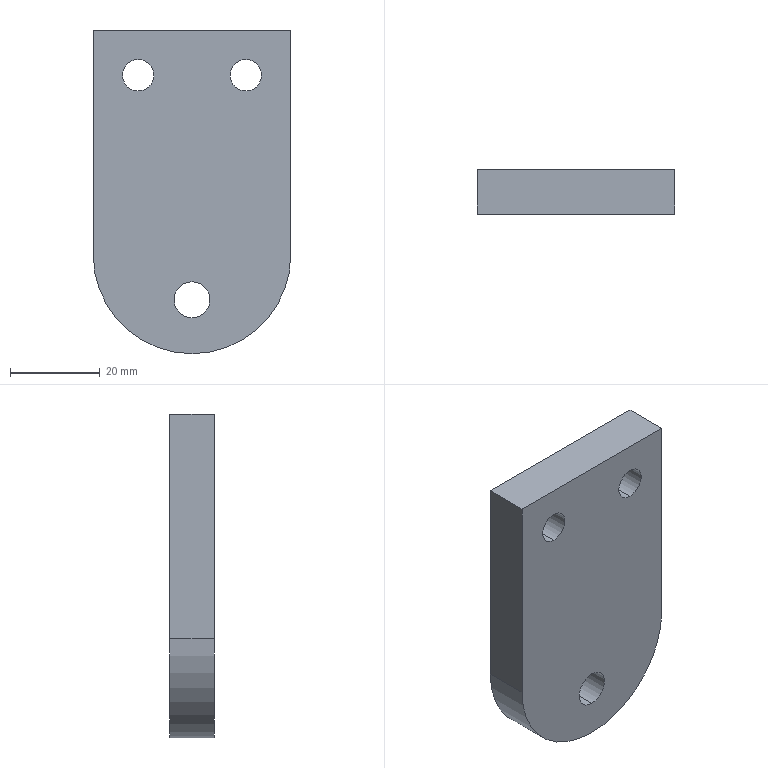Part | STEP file | OP10-146_seal side plate (1) | 1 solid | 13 faces | box 44 x 10 x 72 mm | volume 28330 mm3 | cylinder 8 | plane 5 | commonest cylinder face diameters 7 x4 8 x2 44 x2
STEP:
#1=CARTESIAN_POINT('',(0.,0.,0.));
#2=DIRECTION('',(0.,0.,1.));
#3=DIRECTION('',(1.,0.,0.));
#4=AXIS2_PLACEMENT_3D('',#1,#2,#3);
#5=CARTESIAN_POINT('',(12.,10.,-10.773));
#6=VERTEX_POINT('',#5);
#7=CARTESIAN_POINT('',(12.,0.,-10.773));
#8=VERTEX_POINT('',#7);
#9=CARTESIAN_POINT('',(12.,10.,-10.773));
#10=DIRECTION('',(0.,-1.,0.));
#11=VECTOR('',#10,1.);
#12=LINE('',#9,#11);
#13=CARTESIAN_POINT('',(12.,10.,-7.273));
#14=DIRECTION('',(0.,-1.,0.));
#15=DIRECTION('',(0.,0.,-1.));
#16=AXIS2_PLACEMENT_3D('',#13,#14,#15);
#17=CYLINDRICAL_SURFACE('',#16,3.5);
#18=CARTESIAN_POINT('',(6.283,0.));
#19=DIRECTION('',(0.,1.));
#20=VECTOR('',#19,1.);
#21=LINE('',#18,#20);
#22=(GEOMETRIC_REPRESENTATION_CONTEXT(2)PARAMETRIC_REPRESENTATION_CONTEXT()REPRESENTATION_CONTEXT('',''));
#23=DEFINITIONAL_REPRESENTATION('',(#21),#22);
#24=PCURVE('',#17,#23);
#25=CARTESIAN_POINT('',(12.,10.,-7.273));
#26=DIRECTION('',(0.,-1.,0.));
#27=DIRECTION('',(0.,0.,-1.));
#28=AXIS2_PLACEMENT_3D('',#25,#26,#27);
#29=CYLINDRICAL_SURFACE('',#28,3.5);
#30=CARTESIAN_POINT('',(0.,0.));
#31=DIRECTION('',(0.,1.));
#32=VECTOR('',#31,1.);
#33=LINE('',#30,#32);
#34=(GEOMETRIC_REPRESENTATION_CONTEXT(2)PARAMETRIC_REPRESENTATION_CONTEXT()REPRESENTATION_CONTEXT('',''));
#35=DEFINITIONAL_REPRESENTATION('',(#33),#34);
#36=PCURVE('',#29,#35);
#37=SURFACE_CURVE('',#12,(#24,#36),.PCURVE_S1.);
#38=EDGE_CURVE('',#6,#8,#37,.T.);
#39=ORIENTED_EDGE('',*,*,#38,.T.);
#40=CARTESIAN_POINT('',(12.,0.,-3.773));
#41=VERTEX_POINT('',#40);
#42=CARTESIAN_POINT('',(12.,0.,-7.273));
#43=DIRECTION('',(0.,1.,0.));
#44=DIRECTION('',(0.,0.,1.));
#45=AXIS2_PLACEMENT_3D('',#42,#43,#44);
#46=CIRCLE('',#45,3.5);
#47=CARTESIAN_POINT('',(9.425,10.));
#48=DIRECTION('',(-1.,0.));
#49=VECTOR('',#48,1.);
#50=LINE('',#47,#49);
#51=(GEOMETRIC_REPRESENTATION_CONTEXT(2)PARAMETRIC_REPRESENTATION_CONTEXT()REPRESENTATION_CONTEXT('',''));
#52=DEFINITIONAL_REPRESENTATION('',(#50),#51);
#53=PCURVE('',#17,#52);
#54=CARTESIAN_POINT('',(0.,0.,-47.273));
#55=DIRECTION('',(0.,1.,0.));
#56=DIRECTION('',(0.,0.,1.));
#57=AXIS2_PLACEMENT_3D('',#54,#55,#56);
#58=PLANE('',#57);
#59=CARTESIAN_POINT('',(40.,12.));
#60=DIRECTION('',(1.,0.));
#61=AXIS2_PLACEMENT_2D('',#59,#60);
#62=CIRCLE('',#61,3.5);
#63=(GEOMETRIC_REPRESENTATION_CONTEXT(2)PARAMETRIC_REPRESENTATION_CONTEXT()REPRESENTATION_CONTEXT('',''));
#64=DEFINITIONAL_REPRESENTATION('',(#62),#63);
#65=PCURVE('',#58,#64);
#66=SURFACE_CURVE('',#46,(#53,#65),.PCURVE_S1.);
#67=EDGE_CURVE('',#8,#41,#66,.T.);
#68=ORIENTED_EDGE('',*,*,#67,.T.);
#69=CARTESIAN_POINT('',(12.,10.,-3.773));
#70=VERTEX_POINT('',#69);
#71=CARTESIAN_POINT('',(12.,10.,-3.773));
#72=DIRECTION('',(0.,-1.,0.));
#73=VECTOR('',#72,1.);
#74=LINE('',#71,#73);
#75=CARTESIAN_POINT('',(3.142,0.));
#76=DIRECTION('',(0.,1.));
#77=VECTOR('',#76,1.);
#78=LINE('',#75,#77);
#79=(GEOMETRIC_REPRESENTATION_CONTEXT(2)PARAMETRIC_REPRESENTATION_CONTEXT()REPRESENTATION_CONTEXT('',''));
#80=DEFINITIONAL_REPRESENTATION('',(#78),#79);
#81=PCURVE('',#17,#80);
#82=CARTESIAN_POINT('',(3.142,0.));
#83=DIRECTION('',(0.,1.));
#84=VECTOR('',#83,1.);
#85=LINE('',#82,#84);
#86=(GEOMETRIC_REPRESENTATION_CONTEXT(2)PARAMETRIC_REPRESENTATION_CONTEXT()REPRESENTATION_CONTEXT('',''));
#87=DEFINITIONAL_REPRESENTATION('',(#85),#86);
#88=PCURVE('',#29,#87);
#89=SURFACE_CURVE('',#74,(#81,#88),.PCURVE_S1.);
#90=EDGE_CURVE('',#70,#41,#89,.T.);
#91=ORIENTED_EDGE('',*,*,#90,.F.);
#92=CARTESIAN_POINT('',(12.,10.,-7.273));
#93=DIRECTION('',(0.,1.,0.));
#94=DIRECTION('',(0.,0.,1.));
#95=AXIS2_PLACEMENT_3D('',#92,#93,#94);
#96=CIRCLE('',#95,3.5);
#97=CARTESIAN_POINT('',(9.425,0.));
#98=DIRECTION('',(-1.,0.));
#99=VECTOR('',#98,1.);
#100=LINE('',#97,#99);
#101=(GEOMETRIC_REPRESENTATION_CONTEXT(2)PARAMETRIC_REPRESENTATION_CONTEXT()REPRESENTATION_CONTEXT('',''));
#102=DEFINITIONAL_REPRESENTATION('',(#100),#101);
#103=PCURVE('',#17,#102);
#104=CARTESIAN_POINT('',(0.,10.,-47.273));
#105=DIRECTION('',(0.,1.,0.));
#106=DIRECTION('',(0.,0.,1.));
#107=AXIS2_PLACEMENT_3D('',#104,#105,#106);
#108=PLANE('',#107);
#109=CARTESIAN_POINT('',(40.,12.));
#110=DIRECTION('',(1.,0.));
#111=AXIS2_PLACEMENT_2D('',#109,#110);
#112=CIRCLE('',#111,3.5);
#113=(GEOMETRIC_REPRESENTATION_CONTEXT(2)PARAMETRIC_REPRESENTATION_CONTEXT()REPRESENTATION_CONTEXT('',''));
#114=DEFINITIONAL_REPRESENTATION('',(#112),#113);
#115=PCURVE('',#108,#114);
#116=SURFACE_CURVE('',#96,(#103,#115),.PCURVE_S1.);
#117=EDGE_CURVE('',#6,#70,#116,.T.);
#118=ORIENTED_EDGE('',*,*,#117,.F.);
#119=EDGE_LOOP('',(#39,#68,#91,#118));
#120=FACE_BOUND('',#119,.F.);
#121=ADVANCED_FACE('',(#120),#17,.F.);
#122=CARTESIAN_POINT('',(-12.,10.,-10.773));
#123=VERTEX_POINT('',#122);
#124=CARTESIAN_POINT('',(-12.,0.,-10.773));
#125=VERTEX_POINT('',#124);
#126=CARTESIAN_POINT('',(-12.,10.,-10.773));
#127=DIRECTION('',(0.,-1.,0.));
#128=VECTOR('',#127,1.);
#129=LINE('',#126,#128);
#130=CARTESIAN_POINT('',(-12.,10.,-7.273));
#131=DIRECTION('',(0.,-1.,0.));
#132=DIRECTION('',(0.,0.,-1.));
#133=AXIS2_PLACEMENT_3D('',#130,#131,#132);
#134=CYLINDRICAL_SURFACE('',#133,3.5);
#135=CARTESIAN_POINT('',(6.283,0.));
#136=DIRECTION('',(0.,1.));
#137=VECTOR('',#136,1.);
#138=LINE('',#135,#137);
#139=(GEOMETRIC_REPRESENTATION_CONTEXT(2)PARAMETRIC_REPRESENTATION_CONTEXT()REPRESENTATION_CONTEXT('',''));
#140=DEFINITIONAL_REPRESENTATION('',(#138),#139);
#141=PCURVE('',#134,#140);
#142=CARTESIAN_POINT('',(-12.,10.,-7.273));
#143=DIRECTION('',(0.,-1.,0.));
#144=DIRECTION('',(0.,0.,-1.));
#145=AXIS2_PLACEMENT_3D('',#142,#143,#144);
#146=CYLINDRICAL_SURFACE('',#145,3.5);
#147=CARTESIAN_POINT('',(0.,0.));
#148=DIRECTION('',(0.,1.));
#149=VECTOR('',#148,1.);
#150=LINE('',#147,#149);
#151=(GEOMETRIC_REPRESENTATION_CONTEXT(2)PARAMETRIC_REPRESENTATION_CONTEXT()REPRESENTATION_CONTEXT('',''));
#152=DEFINITIONAL_REPRESENTATION('',(#150),#151);
#153=PCURVE('',#146,#152);
#154=SURFACE_CURVE('',#129,(#141,#153),.PCURVE_S1.);
#155=EDGE_CURVE('',#123,#125,#154,.T.);
#156=ORIENTED_EDGE('',*,*,#155,.T.);
#157=CARTESIAN_POINT('',(-12.,0.,-3.773));
#158=VERTEX_POINT('',#157);
#159=CARTESIAN_POINT('',(-12.,0.,-7.273));
#160=DIRECTION('',(0.,1.,0.));
#161=DIRECTION('',(0.,0.,1.));
#162=AXIS2_PLACEMENT_3D('',#159,#160,#161);
#163=CIRCLE('',#162,3.5);
#164=CARTESIAN_POINT('',(9.425,10.));
#165=DIRECTION('',(-1.,0.));
#166=VECTOR('',#165,1.);
#167=LINE('',#164,#166);
#168=(GEOMETRIC_REPRESENTATION_CONTEXT(2)PARAMETRIC_REPRESENTATION_CONTEXT()REPRESENTATION_CONTEXT('',''));
#169=DEFINITIONAL_REPRESENTATION('',(#167),#168);
#170=PCURVE('',#134,#169);
#171=CARTESIAN_POINT('',(40.,-12.));
#172=DIRECTION('',(1.,0.));
#173=AXIS2_PLACEMENT_2D('',#171,#172);
#174=CIRCLE('',#173,3.5);
#175=(GEOMETRIC_REPRESENTATION_CONTEXT(2)PARAMETRIC_REPRESENTATION_CONTEXT()REPRESENTATION_CONTEXT('',''));
#176=DEFINITIONAL_REPRESENTATION('',(#174),#175);
#177=PCURVE('',#58,#176);
#178=SURFACE_CURVE('',#163,(#170,#177),.PCURVE_S1.);
#179=EDGE_CURVE('',#125,#158,#178,.T.);
#180=ORIENTED_EDGE('',*,*,#179,.T.);
#181=CARTESIAN_POINT('',(-12.,10.,-3.773));
#182=VERTEX_POINT('',#181);
#183=CARTESIAN_POINT('',(-12.,10.,-3.773));
#184=DIRECTION('',(0.,-1.,0.));
#185=VECTOR('',#184,1.);
#186=LINE('',#183,#185);
#187=CARTESIAN_POINT('',(3.142,0.));
#188=DIRECTION('',(0.,1.));
#189=VECTOR('',#188,1.);
#190=LINE('',#187,#189);
#191=(GEOMETRIC_REPRESENTATION_CONTEXT(2)PARAMETRIC_REPRESENTATION_CONTEXT()REPRESENTATION_CONTEXT('',''));
#192=DEFINITIONAL_REPRESENTATION('',(#190),#191);
#193=PCURVE('',#134,#192);
#194=CARTESIAN_POINT('',(3.142,0.));
#195=DIRECTION('',(0.,1.));
#196=VECTOR('',#195,1.);
#197=LINE('',#194,#196);
#198=(GEOMETRIC_REPRESENTATION_CONTEXT(2)PARAMETRIC_REPRESENTATION_CONTEXT()REPRESENTATION_CONTEXT('',''));
#199=DEFINITIONAL_REPRESENTATION('',(#197),#198);
#200=PCURVE('',#146,#199);
#201=SURFACE_CURVE('',#186,(#193,#200),.PCURVE_S1.);
#202=EDGE_CURVE('',#182,#158,#201,.T.);
#203=ORIENTED_EDGE('',*,*,#202,.F.);
#204=CARTESIAN_POINT('',(-12.,10.,-7.273));
#205=DIRECTION('',(0.,1.,0.));
#206=DIRECTION('',(0.,0.,1.));
#207=AXIS2_PLACEMENT_3D('',#204,#205,#206);
#208=CIRCLE('',#207,3.5);
#209=CARTESIAN_POINT('',(9.425,0.));
#210=DIRECTION('',(-1.,0.));
#211=VECTOR('',#210,1.);
#212=LINE('',#209,#211);
#213=(GEOMETRIC_REPRESENTATION_CONTEXT(2)PARAMETRIC_REPRESENTATION_CONTEXT()REPRESENTATION_CONTEXT('',''));
#214=DEFINITIONAL_REPRESENTATION('',(#212),#213);
#215=PCURVE('',#134,#214);
#216=CARTESIAN_POINT('',(40.,-12.));
#217=DIRECTION('',(1.,0.));
#218=AXIS2_PLACEMENT_2D('',#216,#217);
#219=CIRCLE('',#218,3.5);
#220=(GEOMETRIC_REPRESENTATION_CONTEXT(2)PARAMETRIC_REPRESENTATION_CONTEXT()REPRESENTATION_CONTEXT('',''));
#221=DEFINITIONAL_REPRESENTATION('',(#219),#220);
#222=PCURVE('',#108,#221);
#223=SURFACE_CURVE('',#208,(#215,#222),.PCURVE_S1.);
#224=EDGE_CURVE('',#123,#182,#223,.T.);
#225=ORIENTED_EDGE('',*,*,#224,.F.);
#226=EDGE_LOOP('',(#156,#180,#203,#225));
#227=FACE_BOUND('',#226,.F.);
#228=ADVANCED_FACE('',(#227),#134,.F.);
#229=CARTESIAN_POINT('',(0.,10.,-61.273));
#230=VERTEX_POINT('',#229);
#231=CARTESIAN_POINT('',(0.,0.,-61.273));
#232=VERTEX_POINT('',#231);
#233=CARTESIAN_POINT('',(0.,10.,-61.273));
#234=DIRECTION('',(0.,-1.,0.));
#235=VECTOR('',#234,1.);
#236=LINE('',#233,#235);
#237=CARTESIAN_POINT('',(0.,10.,-57.273));
#238=DIRECTION('',(0.,-1.,0.));
#239=DIRECTION('',(0.,0.,-1.));
#240=AXIS2_PLACEMENT_3D('',#237,#238,#239);
#241=CYLINDRICAL_SURFACE('',#240,4.);
#242=CARTESIAN_POINT('',(6.283,0.));
#243=DIRECTION('',(0.,1.));
#244=VECTOR('',#243,1.);
#245=LINE('',#242,#244);
#246=(GEOMETRIC_REPRESENTATION_CONTEXT(2)PARAMETRIC_REPRESENTATION_CONTEXT()REPRESENTATION_CONTEXT('',''));
#247=DEFINITIONAL_REPRESENTATION('',(#245),#246);
#248=PCURVE('',#241,#247);
#249=CARTESIAN_POINT('',(0.,10.,-57.273));
#250=DIRECTION('',(0.,-1.,0.));
#251=DIRECTION('',(0.,0.,-1.));
#252=AXIS2_PLACEMENT_3D('',#249,#250,#251);
#253=CYLINDRICAL_SURFACE('',#252,4.);
#254=CARTESIAN_POINT('',(0.,0.));
#255=DIRECTION('',(0.,1.));
#256=VECTOR('',#255,1.);
#257=LINE('',#254,#256);
#258=(GEOMETRIC_REPRESENTATION_CONTEXT(2)PARAMETRIC_REPRESENTATION_CONTEXT()REPRESENTATION_CONTEXT('',''));
#259=DEFINITIONAL_REPRESENTATION('',(#257),#258);
#260=PCURVE('',#253,#259);
#261=SURFACE_CURVE('',#236,(#248,#260),.PCURVE_S1.);
#262=EDGE_CURVE('',#230,#232,#261,.T.);
#263=ORIENTED_EDGE('',*,*,#262,.T.);
#264=CARTESIAN_POINT('',(0.,0.,-53.273));
#265=VERTEX_POINT('',#264);
#266=CARTESIAN_POINT('',(0.,0.,-57.273));
#267=DIRECTION('',(0.,1.,0.));
#268=DIRECTION('',(0.,0.,1.));
#269=AXIS2_PLACEMENT_3D('',#266,#267,#268);
#270=CIRCLE('',#269,4.);
#271=CARTESIAN_POINT('',(9.425,10.));
#272=DIRECTION('',(-1.,0.));
#273=VECTOR('',#272,1.);
#274=LINE('',#271,#273);
#275=(GEOMETRIC_REPRESENTATION_CONTEXT(2)PARAMETRIC_REPRESENTATION_CONTEXT()REPRESENTATION_CONTEXT('',''));
#276=DEFINITIONAL_REPRESENTATION('',(#274),#275);
#277=PCURVE('',#241,#276);
#278=CARTESIAN_POINT('',(-10.,0.));
#279=DIRECTION('',(1.,0.));
#280=AXIS2_PLACEMENT_2D('',#278,#279);
#281=CIRCLE('',#280,4.);
#282=(GEOMETRIC_REPRESENTATION_CONTEXT(2)PARAMETRIC_REPRESENTATION_CONTEXT()REPRESENTATION_CONTEXT('',''));
#283=DEFINITIONAL_REPRESENTATION('',(#281),#282);
#284=PCURVE('',#58,#283);
#285=SURFACE_CURVE('',#270,(#277,#284),.PCURVE_S1.);
#286=EDGE_CURVE('',#232,#265,#285,.T.);
#287=ORIENTED_EDGE('',*,*,#286,.T.);
#288=CARTESIAN_POINT('',(0.,10.,-53.273));
#289=VERTEX_POINT('',#288);
#290=CARTESIAN_POINT('',(0.,10.,-53.273));
#291=DIRECTION('',(0.,-1.,0.));
#292=VECTOR('',#291,1.);
#293=LINE('',#290,#292);
#294=CARTESIAN_POINT('',(3.142,0.));
#295=DIRECTION('',(0.,1.));
#296=VECTOR('',#295,1.);
#297=LINE('',#294,#296);
#298=(GEOMETRIC_REPRESENTATION_CONTEXT(2)PARAMETRIC_REPRESENTATION_CONTEXT()REPRESENTATION_CONTEXT('',''));
#299=DEFINITIONAL_REPRESENTATION('',(#297),#298);
#300=PCURVE('',#241,#299);
#301=CARTESIAN_POINT('',(3.142,0.));
#302=DIRECTION('',(0.,1.));
#303=VECTOR('',#302,1.);
#304=LINE('',#301,#303);
#305=(GEOMETRIC_REPRESENTATION_CONTEXT(2)PARAMETRIC_REPRESENTATION_CONTEXT()REPRESENTATION_CONTEXT('',''));
#306=DEFINITIONAL_REPRESENTATION('',(#304),#305);
#307=PCURVE('',#253,#306);
#308=SURFACE_CURVE('',#293,(#300,#307),.PCURVE_S1.);
#309=EDGE_CURVE('',#289,#265,#308,.T.);
#310=ORIENTED_EDGE('',*,*,#309,.F.);
#311=CARTESIAN_POINT('',(0.,10.,-57.273));
#312=DIRECTION('',(0.,1.,0.));
#313=DIRECTION('',(0.,0.,1.));
#314=AXIS2_PLACEMENT_3D('',#311,#312,#313);
#315=CIRCLE('',#314,4.);
#316=CARTESIAN_POINT('',(9.425,0.));
#317=DIRECTION('',(-1.,0.));
#318=VECTOR('',#317,1.);
#319=LINE('',#316,#318);
#320=(GEOMETRIC_REPRESENTATION_CONTEXT(2)PARAMETRIC_REPRESENTATION_CONTEXT()REPRESENTATION_CONTEXT('',''));
#321=DEFINITIONAL_REPRESENTATION('',(#319),#320);
#322=PCURVE('',#241,#321);
#323=CARTESIAN_POINT('',(-10.,0.));
#324=DIRECTION('',(1.,0.));
#325=AXIS2_PLACEMENT_2D('',#323,#324);
#326=CIRCLE('',#325,4.);
#327=(GEOMETRIC_REPRESENTATION_CONTEXT(2)PARAMETRIC_REPRESENTATION_CONTEXT()REPRESENTATION_CONTEXT('',''));
#328=DEFINITIONAL_REPRESENTATION('',(#326),#327);
#329=PCURVE('',#108,#328);
#330=SURFACE_CURVE('',#315,(#322,#329),.PCURVE_S1.);
#331=EDGE_CURVE('',#230,#289,#330,.T.);
#332=ORIENTED_EDGE('',*,*,#331,.F.);
#333=EDGE_LOOP('',(#263,#287,#310,#332));
#334=FACE_BOUND('',#333,.F.);
#335=ADVANCED_FACE('',(#334),#241,.F.);
#336=CARTESIAN_POINT('',(0.,10.,-69.273));
#337=VERTEX_POINT('',#336);
#338=CARTESIAN_POINT('',(-22.,10.,-47.273));
#339=VERTEX_POINT('',#338);
#340=CARTESIAN_POINT('',(0.,10.,-47.273));
#341=DIRECTION('',(0.,1.,0.));
#342=DIRECTION('',(0.,0.,1.));
#343=AXIS2_PLACEMENT_3D('',#340,#341,#342);
#344=CIRCLE('',#343,22.);
#345=CARTESIAN_POINT('',(0.,10.,-47.273));
#346=DIRECTION('',(0.,-1.,0.));
#347=DIRECTION('',(0.,0.,-1.));
#348=AXIS2_PLACEMENT_3D('',#345,#346,#347);
#349=CYLINDRICAL_SURFACE('',#348,22.);
#350=CARTESIAN_POINT('',(9.425,0.));
#351=DIRECTION('',(-1.,0.));
#352=VECTOR('',#351,1.);
#353=LINE('',#350,#352);
#354=(GEOMETRIC_REPRESENTATION_CONTEXT(2)PARAMETRIC_REPRESENTATION_CONTEXT()REPRESENTATION_CONTEXT('',''));
#355=DEFINITIONAL_REPRESENTATION('',(#353),#354);
#356=PCURVE('',#349,#355);
#357=CARTESIAN_POINT('',(0.,0.));
#358=DIRECTION('',(1.,0.));
#359=AXIS2_PLACEMENT_2D('',#357,#358);
#360=CIRCLE('',#359,22.);
#361=(GEOMETRIC_REPRESENTATION_CONTEXT(2)PARAMETRIC_REPRESENTATION_CONTEXT()REPRESENTATION_CONTEXT('',''));
#362=DEFINITIONAL_REPRESENTATION('',(#360),#361);
#363=PCURVE('',#108,#362);
#364=SURFACE_CURVE('',#344,(#356,#363),.PCURVE_S1.);
#365=EDGE_CURVE('',#337,#339,#364,.T.);
#366=ORIENTED_EDGE('',*,*,#365,.F.);
#367=CARTESIAN_POINT('',(0.,0.,-69.273));
#368=VERTEX_POINT('',#367);
#369=CARTESIAN_POINT('',(0.,10.,-69.273));
#370=DIRECTION('',(0.,-1.,0.));
#371=VECTOR('',#370,1.);
#372=LINE('',#369,#371);
#373=CARTESIAN_POINT('',(6.283,0.));
#374=DIRECTION('',(0.,1.));
#375=VECTOR('',#374,1.);
#376=LINE('',#373,#375);
#377=(GEOMETRIC_REPRESENTATION_CONTEXT(2)PARAMETRIC_REPRESENTATION_CONTEXT()REPRESENTATION_CONTEXT('',''));
#378=DEFINITIONAL_REPRESENTATION('',(#376),#377);
#379=PCURVE('',#349,#378);
#380=CARTESIAN_POINT('',(0.,10.,-47.273));
#381=DIRECTION('',(0.,-1.,0.));
#382=DIRECTION('',(0.,0.,-1.));
#383=AXIS2_PLACEMENT_3D('',#380,#381,#382);
#384=CYLINDRICAL_SURFACE('',#383,22.);
#385=CARTESIAN_POINT('',(0.,0.));
#386=DIRECTION('',(0.,1.));
#387=VECTOR('',#386,1.);
#388=LINE('',#385,#387);
#389=(GEOMETRIC_REPRESENTATION_CONTEXT(2)PARAMETRIC_REPRESENTATION_CONTEXT()REPRESENTATION_CONTEXT('',''));
#390=DEFINITIONAL_REPRESENTATION('',(#388),#389);
#391=PCURVE('',#384,#390);
#392=SURFACE_CURVE('',#372,(#379,#391),.PCURVE_S1.);
#393=EDGE_CURVE('',#337,#368,#392,.T.);
#394=ORIENTED_EDGE('',*,*,#393,.T.);
#395=CARTESIAN_POINT('',(-22.,0.,-47.273));
#396=VERTEX_POINT('',#395);
#397=CARTESIAN_POINT('',(0.,0.,-47.273));
#398=DIRECTION('',(0.,1.,0.));
#399=DIRECTION('',(0.,0.,1.));
#400=AXIS2_PLACEMENT_3D('',#397,#398,#399);
#401=CIRCLE('',#400,22.);
#402=CARTESIAN_POINT('',(9.425,10.));
#403=DIRECTION('',(-1.,0.));
#404=VECTOR('',#403,1.);
#405=LINE('',#402,#404);
#406=(GEOMETRIC_REPRESENTATION_CONTEXT(2)PARAMETRIC_REPRESENTATION_CONTEXT()REPRESENTATION_CONTEXT('',''));
#407=DEFINITIONAL_REPRESENTATION('',(#405),#406);
#408=PCURVE('',#349,#407);
#409=CARTESIAN_POINT('',(0.,0.));
#410=DIRECTION('',(1.,0.));
#411=AXIS2_PLACEMENT_2D('',#409,#410);
#412=CIRCLE('',#411,22.);
#413=(GEOMETRIC_REPRESENTATION_CONTEXT(2)PARAMETRIC_REPRESENTATION_CONTEXT()REPRESENTATION_CONTEXT('',''));
#414=DEFINITIONAL_REPRESENTATION('',(#412),#413);
#415=PCURVE('',#58,#414);
#416=SURFACE_CURVE('',#401,(#408,#415),.PCURVE_S1.);
#417=EDGE_CURVE('',#368,#396,#416,.T.);
#418=ORIENTED_EDGE('',*,*,#417,.T.);
#419=CARTESIAN_POINT('',(-22.,10.,-47.273));
#420=DIRECTION('',(0.,-1.,0.));
#421=VECTOR('',#420,1.);
#422=LINE('',#419,#421);
#423=CARTESIAN_POINT('',(4.712,0.));
#424=DIRECTION('',(0.,1.));
#425=VECTOR('',#424,1.);
#426=LINE('',#423,#425);
#427=(GEOMETRIC_REPRESENTATION_CONTEXT(2)PARAMETRIC_REPRESENTATION_CONTEXT()REPRESENTATION_CONTEXT('',''));
#428=DEFINITIONAL_REPRESENTATION('',(#426),#427);
#429=PCURVE('',#349,#428);
#430=CARTESIAN_POINT('',(-22.,10.,2.727));
#431=DIRECTION('',(1.,0.,0.));
#432=DIRECTION('',(0.,0.,-1.));
#433=AXIS2_PLACEMENT_3D('',#430,#431,#432);
#434=PLANE('',#433);
#435=CARTESIAN_POINT('',(50.,0.));
#436=DIRECTION('',(0.,-1.));
#437=VECTOR('',#436,1.);
#438=LINE('',#435,#437);
#439=(GEOMETRIC_REPRESENTATION_CONTEXT(2)PARAMETRIC_REPRESENTATION_CONTEXT()REPRESENTATION_CONTEXT('',''));
#440=DEFINITIONAL_REPRESENTATION('',(#438),#439);
#441=PCURVE('',#434,#440);
#442=SURFACE_CURVE('',#422,(#429,#441),.PCURVE_S1.);
#443=EDGE_CURVE('',#339,#396,#442,.T.);
#444=ORIENTED_EDGE('',*,*,#443,.F.);
#445=EDGE_LOOP('',(#366,#394,#418,#444));
#446=FACE_BOUND('',#445,.T.);
#447=ADVANCED_FACE('',(#446),#349,.T.);
#448=ORIENTED_EDGE('',*,*,#224,.F.);
#449=CARTESIAN_POINT('',(-12.,10.,-7.273));
#450=DIRECTION('',(0.,1.,0.));
#451=DIRECTION('',(0.,0.,1.));
#452=AXIS2_PLACEMENT_3D('',#449,#450,#451);
#453=CIRCLE('',#452,3.5);
#454=CARTESIAN_POINT('',(40.,-12.));
#455=DIRECTION('',(1.,0.));
#456=AXIS2_PLACEMENT_2D('',#454,#455);
#457=CIRCLE('',#456,3.5);
#458=(GEOMETRIC_REPRESENTATION_CONTEXT(2)PARAMETRIC_REPRESENTATION_CONTEXT()REPRESENTATION_CONTEXT('',''));
#459=DEFINITIONAL_REPRESENTATION('',(#457),#458);
#460=PCURVE('',#108,#459);
#461=CARTESIAN_POINT('',(3.142,0.));
#462=DIRECTION('',(-1.,0.));
#463=VECTOR('',#462,1.);
#464=LINE('',#461,#463);
#465=(GEOMETRIC_REPRESENTATION_CONTEXT(2)PARAMETRIC_REPRESENTATION_CONTEXT()REPRESENTATION_CONTEXT('',''));
#466=DEFINITIONAL_REPRESENTATION('',(#464),#465);
#467=PCURVE('',#146,#466);
#468=SURFACE_CURVE('',#453,(#460,#467),.PCURVE_S1.);
#469=EDGE_CURVE('',#182,#123,#468,.T.);
#470=ORIENTED_EDGE('',*,*,#469,.F.);
#471=EDGE_LOOP('',(#448,#470));
#472=FACE_BOUND('',#471,.T.);
#473=CARTESIAN_POINT('',(22.,10.,-47.273));
#474=VERTEX_POINT('',#473);
#475=CARTESIAN_POINT('',(0.,10.,-47.273));
#476=DIRECTION('',(0.,1.,0.));
#477=DIRECTION('',(0.,0.,1.));
#478=AXIS2_PLACEMENT_3D('',#475,#476,#477);
#479=CIRCLE('',#478,22.);
#480=CARTESIAN_POINT('',(0.,0.));
#481=DIRECTION('',(1.,0.));
#482=AXIS2_PLACEMENT_2D('',#480,#481);
#483=CIRCLE('',#482,22.);
#484=(GEOMETRIC_REPRESENTATION_CONTEXT(2)PARAMETRIC_REPRESENTATION_CONTEXT()REPRESENTATION_CONTEXT('',''));
#485=DEFINITIONAL_REPRESENTATION('',(#483),#484);
#486=PCURVE('',#108,#485);
#487=CARTESIAN_POINT('',(3.142,0.));
#488=DIRECTION('',(-1.,0.));
#489=VECTOR('',#488,1.);
#490=LINE('',#487,#489);
#491=(GEOMETRIC_REPRESENTATION_CONTEXT(2)PARAMETRIC_REPRESENTATION_CONTEXT()REPRESENTATION_CONTEXT('',''));
#492=DEFINITIONAL_REPRESENTATION('',(#490),#491);
#493=PCURVE('',#384,#492);
#494=SURFACE_CURVE('',#479,(#486,#493),.PCURVE_S1.);
#495=EDGE_CURVE('',#474,#337,#494,.T.);
#496=ORIENTED_EDGE('',*,*,#495,.T.);
#497=ORIENTED_EDGE('',*,*,#365,.T.);
#498=CARTESIAN_POINT('',(-22.,10.,2.727));
#499=VERTEX_POINT('',#498);
#500=CARTESIAN_POINT('',(-22.,10.,2.727));
#501=DIRECTION('',(0.,0.,1.));
#502=VECTOR('',#501,1.);
#503=LINE('',#500,#502);
#504=CARTESIAN_POINT('',(50.,-22.));
#505=DIRECTION('',(1.,0.));
#506=VECTOR('',#505,1.);
#507=LINE('',#504,#506);
#508=(GEOMETRIC_REPRESENTATION_CONTEXT(2)PARAMETRIC_REPRESENTATION_CONTEXT()REPRESENTATION_CONTEXT('',''));
#509=DEFINITIONAL_REPRESENTATION('',(#507),#508);
#510=PCURVE('',#108,#509);
#511=CARTESIAN_POINT('',(0.,0.));
#512=DIRECTION('',(-1.,0.));
#513=VECTOR('',#512,1.);
#514=LINE('',#511,#513);
#515=(GEOMETRIC_REPRESENTATION_CONTEXT(2)PARAMETRIC_REPRESENTATION_CONTEXT()REPRESENTATION_CONTEXT('',''));
#516=DEFINITIONAL_REPRESENTATION('',(#514),#515);
#517=PCURVE('',#434,#516);
#518=SURFACE_CURVE('',#503,(#510,#517),.PCURVE_S1.);
#519=EDGE_CURVE('',#339,#499,#518,.T.);
#520=ORIENTED_EDGE('',*,*,#519,.T.);
#521=CARTESIAN_POINT('',(22.,10.,2.727));
#522=VERTEX_POINT('',#521);
#523=CARTESIAN_POINT('',(-22.,10.,2.727));
#524=DIRECTION('',(1.,0.,0.));
#525=VECTOR('',#524,1.);
#526=LINE('',#523,#525);
#527=CARTESIAN_POINT('',(50.,-22.));
#528=DIRECTION('',(0.,1.));
#529=VECTOR('',#528,1.);
#530=LINE('',#527,#529);
#531=(GEOMETRIC_REPRESENTATION_CONTEXT(2)PARAMETRIC_REPRESENTATION_CONTEXT()REPRESENTATION_CONTEXT('',''));
#532=DEFINITIONAL_REPRESENTATION('',(#530),#531);
#533=PCURVE('',#108,#532);
#534=CARTESIAN_POINT('',(-22.,10.,2.727));
#535=DIRECTION('',(0.,0.,-1.));
#536=DIRECTION('',(-1.,0.,0.));
#537=AXIS2_PLACEMENT_3D('',#534,#535,#536);
#538=PLANE('',#537);
#539=CARTESIAN_POINT('',(0.,0.));
#540=DIRECTION('',(-1.,0.));
#541=VECTOR('',#540,1.);
#542=LINE('',#539,#541);
#543=(GEOMETRIC_REPRESENTATION_CONTEXT(2)PARAMETRIC_REPRESENTATION_CONTEXT()REPRESENTATION_CONTEXT('',''));
#544=DEFINITIONAL_REPRESENTATION('',(#542),#543);
#545=PCURVE('',#538,#544);
#546=SURFACE_CURVE('',#526,(#533,#545),.PCURVE_S1.);
#547=EDGE_CURVE('',#499,#522,#546,.T.);
#548=ORIENTED_EDGE('',*,*,#547,.T.);
#549=CARTESIAN_POINT('',(22.,10.,2.727));
#550=DIRECTION('',(0.,0.,-1.));
#551=VECTOR('',#550,1.);
#552=LINE('',#549,#551);
#553=CARTESIAN_POINT('',(50.,22.));
#554=DIRECTION('',(-1.,0.));
#555=VECTOR('',#554,1.);
#556=LINE('',#553,#555);
#557=(GEOMETRIC_REPRESENTATION_CONTEXT(2)PARAMETRIC_REPRESENTATION_CONTEXT()REPRESENTATION_CONTEXT('',''));
#558=DEFINITIONAL_REPRESENTATION('',(#556),#557);
#559=PCURVE('',#108,#558);
#560=CARTESIAN_POINT('',(22.,10.,2.727));
#561=DIRECTION('',(-1.,0.,0.));
#562=DIRECTION('',(0.,0.,1.));
#563=AXIS2_PLACEMENT_3D('',#560,#561,#562);
#564=PLANE('',#563);
#565=CARTESIAN_POINT('',(0.,0.));
#566=DIRECTION('',(-1.,0.));
#567=VECTOR('',#566,1.);
#568=LINE('',#565,#567);
#569=(GEOMETRIC_REPRESENTATION_CONTEXT(2)PARAMETRIC_REPRESENTATION_CONTEXT()REPRESENTATION_CONTEXT('',''));
#570=DEFINITIONAL_REPRESENTATION('',(#568),#569);
#571=PCURVE('',#564,#570);
#572=SURFACE_CURVE('',#552,(#559,#571),.PCURVE_S1.);
#573=EDGE_CURVE('',#522,#474,#572,.T.);
#574=ORIENTED_EDGE('',*,*,#573,.T.);
#575=EDGE_LOOP('',(#496,#497,#520,#548,#574));
#576=FACE_BOUND('',#575,.T.);
#577=ORIENTED_EDGE('',*,*,#331,.F.);
#578=CARTESIAN_POINT('',(0.,10.,-57.273));
#579=DIRECTION('',(0.,1.,0.));
#580=DIRECTION('',(0.,0.,1.));
#581=AXIS2_PLACEMENT_3D('',#578,#579,#580);
#582=CIRCLE('',#581,4.);
#583=CARTESIAN_POINT('',(-10.,0.));
#584=DIRECTION('',(1.,0.));
#585=AXIS2_PLACEMENT_2D('',#583,#584);
#586=CIRCLE('',#585,4.);
#587=(GEOMETRIC_REPRESENTATION_CONTEXT(2)PARAMETRIC_REPRESENTATION_CONTEXT()REPRESENTATION_CONTEXT('',''));
#588=DEFINITIONAL_REPRESENTATION('',(#586),#587);
#589=PCURVE('',#108,#588);
#590=CARTESIAN_POINT('',(3.142,0.));
#591=DIRECTION('',(-1.,0.));
#592=VECTOR('',#591,1.);
#593=LINE('',#590,#592);
#594=(GEOMETRIC_REPRESENTATION_CONTEXT(2)PARAMETRIC_REPRESENTATION_CONTEXT()REPRESENTATION_CONTEXT('',''));
#595=DEFINITIONAL_REPRESENTATION('',(#593),#594);
#596=PCURVE('',#253,#595);
#597=SURFACE_CURVE('',#582,(#589,#596),.PCURVE_S1.);
#598=EDGE_CURVE('',#289,#230,#597,.T.);
#599=ORIENTED_EDGE('',*,*,#598,.F.);
#600=EDGE_LOOP('',(#577,#599));
#601=FACE_BOUND('',#600,.T.);
#602=ORIENTED_EDGE('',*,*,#117,.F.);
#603=CARTESIAN_POINT('',(12.,10.,-7.273));
#604=DIRECTION('',(0.,1.,0.));
#605=DIRECTION('',(0.,0.,1.));
#606=AXIS2_PLACEMENT_3D('',#603,#604,#605);
#607=CIRCLE('',#606,3.5);
#608=CARTESIAN_POINT('',(40.,12.));
#609=DIRECTION('',(1.,0.));
#610=AXIS2_PLACEMENT_2D('',#608,#609);
#611=CIRCLE('',#610,3.5);
#612=(GEOMETRIC_REPRESENTATION_CONTEXT(2)PARAMETRIC_REPRESENTATION_CONTEXT()REPRESENTATION_CONTEXT('',''));
#613=DEFINITIONAL_REPRESENTATION('',(#611),#612);
#614=PCURVE('',#108,#613);
#615=CARTESIAN_POINT('',(3.142,0.));
#616=DIRECTION('',(-1.,0.));
#617=VECTOR('',#616,1.);
#618=LINE('',#615,#617);
#619=(GEOMETRIC_REPRESENTATION_CONTEXT(2)PARAMETRIC_REPRESENTATION_CONTEXT()REPRESENTATION_CONTEXT('',''));
#620=DEFINITIONAL_REPRESENTATION('',(#618),#619);
#621=PCURVE('',#29,#620);
#622=SURFACE_CURVE('',#607,(#614,#621),.PCURVE_S1.);
#623=EDGE_CURVE('',#70,#6,#622,.T.);
#624=ORIENTED_EDGE('',*,*,#623,.F.);
#625=EDGE_LOOP('',(#602,#624));
#626=FACE_BOUND('',#625,.T.);
#627=ADVANCED_FACE('',(#472,#576,#601,#626),#108,.T.);
#628=ORIENTED_EDGE('',*,*,#179,.T.);
#629=CARTESIAN_POINT('',(-12.,0.,-7.273));
#630=DIRECTION('',(0.,1.,0.));
#631=DIRECTION('',(0.,0.,1.));
#632=AXIS2_PLACEMENT_3D('',#629,#630,#631);
#633=CIRCLE('',#632,3.5);
#634=CARTESIAN_POINT('',(40.,-12.));
#635=DIRECTION('',(1.,0.));
#636=AXIS2_PLACEMENT_2D('',#634,#635);
#637=CIRCLE('',#636,3.5);
#638=(GEOMETRIC_REPRESENTATION_CONTEXT(2)PARAMETRIC_REPRESENTATION_CONTEXT()REPRESENTATION_CONTEXT('',''));
#639=DEFINITIONAL_REPRESENTATION('',(#637),#638);
#640=PCURVE('',#58,#639);
#641=CARTESIAN_POINT('',(3.142,10.));
#642=DIRECTION('',(-1.,0.));
#643=VECTOR('',#642,1.);
#644=LINE('',#641,#643);
#645=(GEOMETRIC_REPRESENTATION_CONTEXT(2)PARAMETRIC_REPRESENTATION_CONTEXT()REPRESENTATION_CONTEXT('',''));
#646=DEFINITIONAL_REPRESENTATION('',(#644),#645);
#647=PCURVE('',#146,#646);
#648=SURFACE_CURVE('',#633,(#640,#647),.PCURVE_S1.);
#649=EDGE_CURVE('',#158,#125,#648,.T.);
#650=ORIENTED_EDGE('',*,*,#649,.T.);
#651=EDGE_LOOP('',(#628,#650));
#652=FACE_BOUND('',#651,.T.);
#653=CARTESIAN_POINT('',(22.,0.,-47.273));
#654=VERTEX_POINT('',#653);
#655=CARTESIAN_POINT('',(0.,0.,-47.273));
#656=DIRECTION('',(0.,1.,0.));
#657=DIRECTION('',(0.,0.,1.));
#658=AXIS2_PLACEMENT_3D('',#655,#656,#657);
#659=CIRCLE('',#658,22.);
#660=CARTESIAN_POINT('',(0.,0.));
#661=DIRECTION('',(1.,0.));
#662=AXIS2_PLACEMENT_2D('',#660,#661);
#663=CIRCLE('',#662,22.);
#664=(GEOMETRIC_REPRESENTATION_CONTEXT(2)PARAMETRIC_REPRESENTATION_CONTEXT()REPRESENTATION_CONTEXT('',''));
#665=DEFINITIONAL_REPRESENTATION('',(#663),#664);
#666=PCURVE('',#58,#665);
#667=CARTESIAN_POINT('',(3.142,10.));
#668=DIRECTION('',(-1.,0.));
#669=VECTOR('',#668,1.);
#670=LINE('',#667,#669);
#671=(GEOMETRIC_REPRESENTATION_CONTEXT(2)PARAMETRIC_REPRESENTATION_CONTEXT()REPRESENTATION_CONTEXT('',''));
#672=DEFINITIONAL_REPRESENTATION('',(#670),#671);
#673=PCURVE('',#384,#672);
#674=SURFACE_CURVE('',#659,(#666,#673),.PCURVE_S1.);
#675=EDGE_CURVE('',#654,#368,#674,.T.);
#676=ORIENTED_EDGE('',*,*,#675,.F.);
#677=CARTESIAN_POINT('',(22.,0.,2.727));
#678=VERTEX_POINT('',#677);
#679=CARTESIAN_POINT('',(22.,0.,2.727));
#680=DIRECTION('',(0.,0.,-1.));
#681=VECTOR('',#680,1.);
#682=LINE('',#679,#681);
#683=CARTESIAN_POINT('',(50.,22.));
#684=DIRECTION('',(-1.,0.));
#685=VECTOR('',#684,1.);
#686=LINE('',#683,#685);
#687=(GEOMETRIC_REPRESENTATION_CONTEXT(2)PARAMETRIC_REPRESENTATION_CONTEXT()REPRESENTATION_CONTEXT('',''));
#688=DEFINITIONAL_REPRESENTATION('',(#686),#687);
#689=PCURVE('',#58,#688);
#690=CARTESIAN_POINT('',(0.,-10.));
#691=DIRECTION('',(-1.,0.));
#692=VECTOR('',#691,1.);
#693=LINE('',#690,#692);
#694=(GEOMETRIC_REPRESENTATION_CONTEXT(2)PARAMETRIC_REPRESENTATION_CONTEXT()REPRESENTATION_CONTEXT('',''));
#695=DEFINITIONAL_REPRESENTATION('',(#693),#694);
#696=PCURVE('',#564,#695);
#697=SURFACE_CURVE('',#682,(#689,#696),.PCURVE_S1.);
#698=EDGE_CURVE('',#678,#654,#697,.T.);
#699=ORIENTED_EDGE('',*,*,#698,.F.);
#700=CARTESIAN_POINT('',(-22.,0.,2.727));
#701=VERTEX_POINT('',#700);
#702=CARTESIAN_POINT('',(-22.,0.,2.727));
#703=DIRECTION('',(1.,0.,0.));
#704=VECTOR('',#703,1.);
#705=LINE('',#702,#704);
#706=CARTESIAN_POINT('',(50.,-22.));
#707=DIRECTION('',(0.,1.));
#708=VECTOR('',#707,1.);
#709=LINE('',#706,#708);
#710=(GEOMETRIC_REPRESENTATION_CONTEXT(2)PARAMETRIC_REPRESENTATION_CONTEXT()REPRESENTATION_CONTEXT('',''));
#711=DEFINITIONAL_REPRESENTATION('',(#709),#710);
#712=PCURVE('',#58,#711);
#713=CARTESIAN_POINT('',(0.,-10.));
#714=DIRECTION('',(-1.,0.));
#715=VECTOR('',#714,1.);
#716=LINE('',#713,#715);
#717=(GEOMETRIC_REPRESENTATION_CONTEXT(2)PARAMETRIC_REPRESENTATION_CONTEXT()REPRESENTATION_CONTEXT('',''));
#718=DEFINITIONAL_REPRESENTATION('',(#716),#717);
#719=PCURVE('',#538,#718);
#720=SURFACE_CURVE('',#705,(#712,#719),.PCURVE_S1.);
#721=EDGE_CURVE('',#701,#678,#720,.T.);
#722=ORIENTED_EDGE('',*,*,#721,.F.);
#723=CARTESIAN_POINT('',(-22.,0.,2.727));
#724=DIRECTION('',(0.,0.,1.));
#725=VECTOR('',#724,1.);
#726=LINE('',#723,#725);
#727=CARTESIAN_POINT('',(50.,-22.));
#728=DIRECTION('',(1.,0.));
#729=VECTOR('',#728,1.);
#730=LINE('',#727,#729);
#731=(GEOMETRIC_REPRESENTATION_CONTEXT(2)PARAMETRIC_REPRESENTATION_CONTEXT()REPRESENTATION_CONTEXT('',''));
#732=DEFINITIONAL_REPRESENTATION('',(#730),#731);
#733=PCURVE('',#58,#732);
#734=CARTESIAN_POINT('',(0.,-10.));
#735=DIRECTION('',(-1.,0.));
#736=VECTOR('',#735,1.);
#737=LINE('',#734,#736);
#738=(GEOMETRIC_REPRESENTATION_CONTEXT(2)PARAMETRIC_REPRESENTATION_CONTEXT()REPRESENTATION_CONTEXT('',''));
#739=DEFINITIONAL_REPRESENTATION('',(#737),#738);
#740=PCURVE('',#434,#739);
#741=SURFACE_CURVE('',#726,(#733,#740),.PCURVE_S1.);
#742=EDGE_CURVE('',#396,#701,#741,.T.);
#743=ORIENTED_EDGE('',*,*,#742,.F.);
#744=ORIENTED_EDGE('',*,*,#417,.F.);
#745=EDGE_LOOP('',(#676,#699,#722,#743,#744));
#746=FACE_BOUND('',#745,.T.);
#747=ORIENTED_EDGE('',*,*,#286,.T.);
#748=CARTESIAN_POINT('',(0.,0.,-57.273));
#749=DIRECTION('',(0.,1.,0.));
#750=DIRECTION('',(0.,0.,1.));
#751=AXIS2_PLACEMENT_3D('',#748,#749,#750);
#752=CIRCLE('',#751,4.);
#753=CARTESIAN_POINT('',(-10.,0.));
#754=DIRECTION('',(1.,0.));
#755=AXIS2_PLACEMENT_2D('',#753,#754);
#756=CIRCLE('',#755,4.);
#757=(GEOMETRIC_REPRESENTATION_CONTEXT(2)PARAMETRIC_REPRESENTATION_CONTEXT()REPRESENTATION_CONTEXT('',''));
#758=DEFINITIONAL_REPRESENTATION('',(#756),#757);
#759=PCURVE('',#58,#758);
#760=CARTESIAN_POINT('',(3.142,10.));
#761=DIRECTION('',(-1.,0.));
#762=VECTOR('',#761,1.);
#763=LINE('',#760,#762);
#764=(GEOMETRIC_REPRESENTATION_CONTEXT(2)PARAMETRIC_REPRESENTATION_CONTEXT()REPRESENTATION_CONTEXT('',''));
#765=DEFINITIONAL_REPRESENTATION('',(#763),#764);
#766=PCURVE('',#253,#765);
#767=SURFACE_CURVE('',#752,(#759,#766),.PCURVE_S1.);
#768=EDGE_CURVE('',#265,#232,#767,.T.);
#769=ORIENTED_EDGE('',*,*,#768,.T.);
#770=EDGE_LOOP('',(#747,#769));
#771=FACE_BOUND('',#770,.T.);
#772=ORIENTED_EDGE('',*,*,#67,.T.);
#773=CARTESIAN_POINT('',(12.,0.,-7.273));
#774=DIRECTION('',(0.,1.,0.));
#775=DIRECTION('',(0.,0.,1.));
#776=AXIS2_PLACEMENT_3D('',#773,#774,#775);
#777=CIRCLE('',#776,3.5);
#778=CARTESIAN_POINT('',(40.,12.));
#779=DIRECTION('',(1.,0.));
#780=AXIS2_PLACEMENT_2D('',#778,#779);
#781=CIRCLE('',#780,3.5);
#782=(GEOMETRIC_REPRESENTATION_CONTEXT(2)PARAMETRIC_REPRESENTATION_CONTEXT()REPRESENTATION_CONTEXT('',''));
#783=DEFINITIONAL_REPRESENTATION('',(#781),#782);
#784=PCURVE('',#58,#783);
#785=CARTESIAN_POINT('',(3.142,10.));
#786=DIRECTION('',(-1.,0.));
#787=VECTOR('',#786,1.);
#788=LINE('',#785,#787);
#789=(GEOMETRIC_REPRESENTATION_CONTEXT(2)PARAMETRIC_REPRESENTATION_CONTEXT()REPRESENTATION_CONTEXT('',''));
#790=DEFINITIONAL_REPRESENTATION('',(#788),#789);
#791=PCURVE('',#29,#790);
#792=SURFACE_CURVE('',#777,(#784,#791),.PCURVE_S1.);
#793=EDGE_CURVE('',#41,#8,#792,.T.);
#794=ORIENTED_EDGE('',*,*,#793,.T.);
#795=EDGE_LOOP('',(#772,#794));
#796=FACE_BOUND('',#795,.T.);
#797=ADVANCED_FACE('',(#652,#746,#771,#796),#58,.F.);
#798=ORIENTED_EDGE('',*,*,#393,.F.);
#799=ORIENTED_EDGE('',*,*,#495,.F.);
#800=CARTESIAN_POINT('',(22.,10.,-47.273));
#801=DIRECTION('',(0.,-1.,0.));
#802=VECTOR('',#801,1.);
#803=LINE('',#800,#802);
#804=CARTESIAN_POINT('',(1.571,0.));
#805=DIRECTION('',(0.,1.));
#806=VECTOR('',#805,1.);
#807=LINE('',#804,#806);
#808=(GEOMETRIC_REPRESENTATION_CONTEXT(2)PARAMETRIC_REPRESENTATION_CONTEXT()REPRESENTATION_CONTEXT('',''));
#809=DEFINITIONAL_REPRESENTATION('',(#807),#808);
#810=PCURVE('',#384,#809);
#811=CARTESIAN_POINT('',(-50.,0.));
#812=DIRECTION('',(0.,-1.));
#813=VECTOR('',#812,1.);
#814=LINE('',#811,#813);
#815=(GEOMETRIC_REPRESENTATION_CONTEXT(2)PARAMETRIC_REPRESENTATION_CONTEXT()REPRESENTATION_CONTEXT('',''));
#816=DEFINITIONAL_REPRESENTATION('',(#814),#815);
#817=PCURVE('',#564,#816);
#818=SURFACE_CURVE('',#803,(#810,#817),.PCURVE_S1.);
#819=EDGE_CURVE('',#474,#654,#818,.T.);
#820=ORIENTED_EDGE('',*,*,#819,.T.);
#821=ORIENTED_EDGE('',*,*,#675,.T.);
#822=EDGE_LOOP('',(#798,#799,#820,#821));
#823=FACE_BOUND('',#822,.T.);
#824=ADVANCED_FACE('',(#823),#384,.T.);
#825=ORIENTED_EDGE('',*,*,#742,.T.);
#826=CARTESIAN_POINT('',(-22.,10.,2.727));
#827=DIRECTION('',(0.,-1.,0.));
#828=VECTOR('',#827,1.);
#829=LINE('',#826,#828);
#830=CARTESIAN_POINT('',(0.,0.));
#831=DIRECTION('',(0.,-1.));
#832=VECTOR('',#831,1.);
#833=LINE('',#830,#832);
#834=(GEOMETRIC_REPRESENTATION_CONTEXT(2)PARAMETRIC_REPRESENTATION_CONTEXT()REPRESENTATION_CONTEXT('',''));
#835=DEFINITIONAL_REPRESENTATION('',(#833),#834);
#836=PCURVE('',#434,#835);
#837=CARTESIAN_POINT('',(0.,0.));
#838=DIRECTION('',(0.,-1.));
#839=VECTOR('',#838,1.);
#840=LINE('',#837,#839);
#841=(GEOMETRIC_REPRESENTATION_CONTEXT(2)PARAMETRIC_REPRESENTATION_CONTEXT()REPRESENTATION_CONTEXT('',''));
#842=DEFINITIONAL_REPRESENTATION('',(#840),#841);
#843=PCURVE('',#538,#842);
#844=SURFACE_CURVE('',#829,(#836,#843),.PCURVE_S1.);
#845=EDGE_CURVE('',#499,#701,#844,.T.);
#846=ORIENTED_EDGE('',*,*,#845,.F.);
#847=ORIENTED_EDGE('',*,*,#519,.F.);
#848=ORIENTED_EDGE('',*,*,#443,.T.);
#849=EDGE_LOOP('',(#825,#846,#847,#848));
#850=FACE_BOUND('',#849,.T.);
#851=ADVANCED_FACE('',(#850),#434,.F.);
#852=ORIENTED_EDGE('',*,*,#721,.T.);
#853=CARTESIAN_POINT('',(22.,10.,2.727));
#854=DIRECTION('',(0.,-1.,0.));
#855=VECTOR('',#854,1.);
#856=LINE('',#853,#855);
#857=CARTESIAN_POINT('',(-44.,0.));
#858=DIRECTION('',(0.,-1.));
#859=VECTOR('',#858,1.);
#860=LINE('',#857,#859);
#861=(GEOMETRIC_REPRESENTATION_CONTEXT(2)PARAMETRIC_REPRESENTATION_CONTEXT()REPRESENTATION_CONTEXT('',''));
#862=DEFINITIONAL_REPRESENTATION('',(#860),#861);
#863=PCURVE('',#538,#862);
#864=CARTESIAN_POINT('',(0.,0.));
#865=DIRECTION('',(0.,-1.));
#866=VECTOR('',#865,1.);
#867=LINE('',#864,#866);
#868=(GEOMETRIC_REPRESENTATION_CONTEXT(2)PARAMETRIC_REPRESENTATION_CONTEXT()REPRESENTATION_CONTEXT('',''));
#869=DEFINITIONAL_REPRESENTATION('',(#867),#868);
#870=PCURVE('',#564,#869);
#871=SURFACE_CURVE('',#856,(#863,#870),.PCURVE_S1.);
#872=EDGE_CURVE('',#522,#678,#871,.T.);
#873=ORIENTED_EDGE('',*,*,#872,.F.);
#874=ORIENTED_EDGE('',*,*,#547,.F.);
#875=ORIENTED_EDGE('',*,*,#845,.T.);
#876=EDGE_LOOP('',(#852,#873,#874,#875));
#877=FACE_BOUND('',#876,.T.);
#878=ADVANCED_FACE('',(#877),#538,.F.);
#879=ORIENTED_EDGE('',*,*,#698,.T.);
#880=ORIENTED_EDGE('',*,*,#819,.F.);
#881=ORIENTED_EDGE('',*,*,#573,.F.);
#882=ORIENTED_EDGE('',*,*,#872,.T.);
#883=EDGE_LOOP('',(#879,#880,#881,#882));
#884=FACE_BOUND('',#883,.T.);
#885=ADVANCED_FACE('',(#884),#564,.F.);
#886=ORIENTED_EDGE('',*,*,#768,.T.);
#887=ORIENTED_EDGE('',*,*,#262,.F.);
#888=ORIENTED_EDGE('',*,*,#598,.F.);
#889=ORIENTED_EDGE('',*,*,#309,.T.);
#890=EDGE_LOOP('',(#886,#887,#888,#889));
#891=FACE_BOUND('',#890,.F.);
#892=ADVANCED_FACE('',(#891),#253,.F.);
#893=ORIENTED_EDGE('',*,*,#649,.T.);
#894=ORIENTED_EDGE('',*,*,#155,.F.);
#895=ORIENTED_EDGE('',*,*,#469,.F.);
#896=ORIENTED_EDGE('',*,*,#202,.T.);
#897=EDGE_LOOP('',(#893,#894,#895,#896));
#898=FACE_BOUND('',#897,.F.);
#899=ADVANCED_FACE('',(#898),#146,.F.);
#900=ORIENTED_EDGE('',*,*,#793,.T.);
#901=ORIENTED_EDGE('',*,*,#38,.F.);
#902=ORIENTED_EDGE('',*,*,#623,.F.);
#903=ORIENTED_EDGE('',*,*,#90,.T.);
#904=EDGE_LOOP('',(#900,#901,#902,#903));
#905=FACE_BOUND('',#904,.F.);
#906=ADVANCED_FACE('',(#905),#29,.F.);
#907=CLOSED_SHELL('',(#121,#228,#335,#447,#627,#797,#824,#851,#878,#885,#892,#899,#906));
#908=MANIFOLD_SOLID_BREP('',#907);
#909=(LENGTH_UNIT()NAMED_UNIT(*)SI_UNIT(.MILLI.,.METRE.));
#910=UNCERTAINTY_MEASURE_WITH_UNIT(LENGTH_MEASURE(0.0000001),#909,'','');
#911=(NAMED_UNIT(*)PLANE_ANGLE_UNIT()SI_UNIT($,.RADIAN.));
#912=(NAMED_UNIT(*)SI_UNIT($,.STERADIAN.)SOLID_ANGLE_UNIT());
#913=(GEOMETRIC_REPRESENTATION_CONTEXT(3)GLOBAL_UNCERTAINTY_ASSIGNED_CONTEXT((#910))GLOBAL_UNIT_ASSIGNED_CONTEXT((#909,#911,#912))REPRESENTATION_CONTEXT('',''));
#914=ADVANCED_BREP_SHAPE_REPRESENTATION('',(#4,#908),#913);